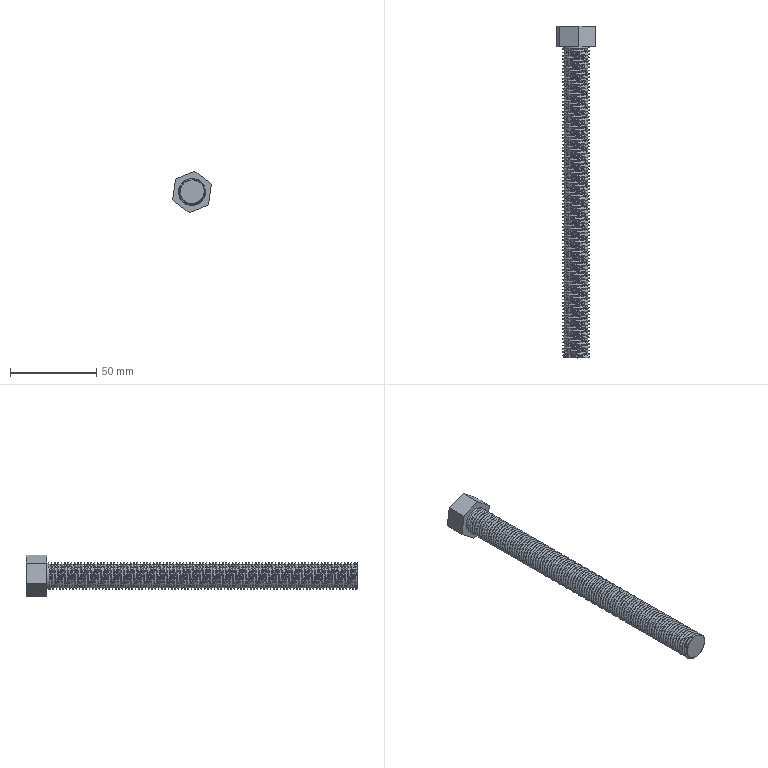Part | STEP file | Scale factor 1[12] | 1 solid | 203 faces | box 22.481 x 192.001 x 24.013 mm | volume 34227 mm3 | cylinder 190 | plane 10 | spline 3 | commonest cylinder face diameters 15.6 x190